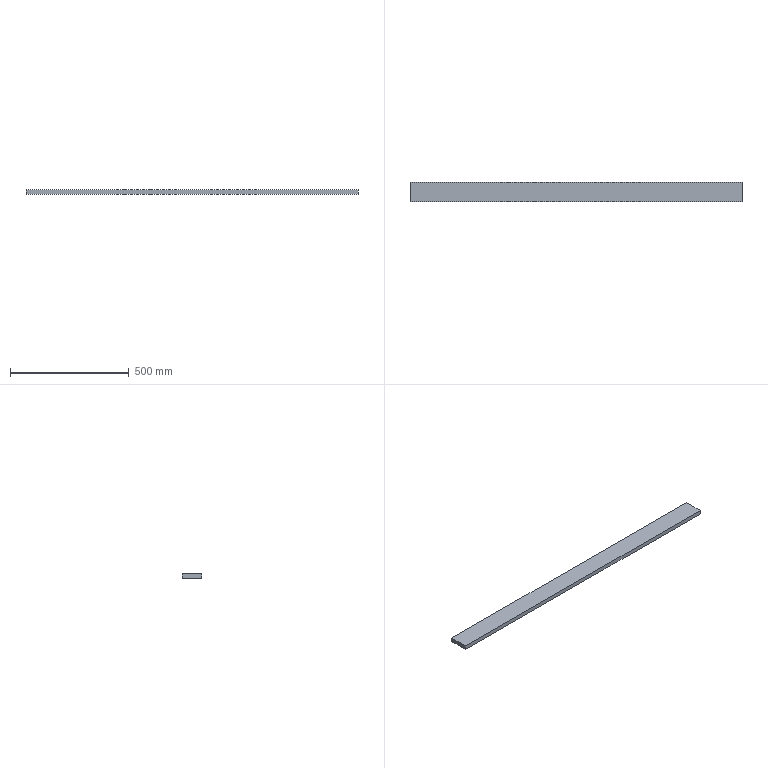Part | STEP file | Frame_right | 1 solid | 6 faces | box 1400 x 82 x 18 mm | volume 2066400 mm3 | plane 6
STEP:
#1=CARTESIAN_POINT('',(0.,0.,0.));
#2=DIRECTION('',(0.,0.,1.));
#3=DIRECTION('',(1.,0.,0.));
#4=AXIS2_PLACEMENT_3D('',#1,#2,#3);
#5=CARTESIAN_POINT('',(-700.,41.,0.));
#6=VERTEX_POINT('',#5);
#7=CARTESIAN_POINT('',(-700.,41.,18.));
#8=VERTEX_POINT('',#7);
#9=CARTESIAN_POINT('',(-700.,41.,0.));
#10=DIRECTION('',(0.,0.,1.));
#11=VECTOR('',#10,1.);
#12=LINE('',#9,#11);
#13=CARTESIAN_POINT('',(-700.,41.,0.));
#14=DIRECTION('',(1.,0.,0.));
#15=DIRECTION('',(0.,-1.,0.));
#16=AXIS2_PLACEMENT_3D('',#13,#14,#15);
#17=PLANE('',#16);
#18=CARTESIAN_POINT('',(0.,0.));
#19=DIRECTION('',(0.,-1.));
#20=VECTOR('',#19,1.);
#21=LINE('',#18,#20);
#22=(GEOMETRIC_REPRESENTATION_CONTEXT(2)PARAMETRIC_REPRESENTATION_CONTEXT()REPRESENTATION_CONTEXT('',''));
#23=DEFINITIONAL_REPRESENTATION('',(#21),#22);
#24=PCURVE('',#17,#23);
#25=CARTESIAN_POINT('',(700.,41.,0.));
#26=DIRECTION('',(0.,-1.,0.));
#27=DIRECTION('',(-1.,0.,0.));
#28=AXIS2_PLACEMENT_3D('',#25,#26,#27);
#29=PLANE('',#28);
#30=CARTESIAN_POINT('',(1400.,0.));
#31=DIRECTION('',(0.,-1.));
#32=VECTOR('',#31,1.);
#33=LINE('',#30,#32);
#34=(GEOMETRIC_REPRESENTATION_CONTEXT(2)PARAMETRIC_REPRESENTATION_CONTEXT()REPRESENTATION_CONTEXT('',''));
#35=DEFINITIONAL_REPRESENTATION('',(#33),#34);
#36=PCURVE('',#29,#35);
#37=SURFACE_CURVE('',#12,(#24,#36),.PCURVE_S1.);
#38=EDGE_CURVE('',#6,#8,#37,.T.);
#39=ORIENTED_EDGE('',*,*,#38,.T.);
#40=CARTESIAN_POINT('',(-700.,-41.,18.));
#41=VERTEX_POINT('',#40);
#42=CARTESIAN_POINT('',(-700.,41.,18.));
#43=DIRECTION('',(0.,-1.,0.));
#44=VECTOR('',#43,1.);
#45=LINE('',#42,#44);
#46=CARTESIAN_POINT('',(0.,-18.));
#47=DIRECTION('',(1.,0.));
#48=VECTOR('',#47,1.);
#49=LINE('',#46,#48);
#50=(GEOMETRIC_REPRESENTATION_CONTEXT(2)PARAMETRIC_REPRESENTATION_CONTEXT()REPRESENTATION_CONTEXT('',''));
#51=DEFINITIONAL_REPRESENTATION('',(#49),#50);
#52=PCURVE('',#17,#51);
#53=CARTESIAN_POINT('',(0.,0.,18.));
#54=DIRECTION('',(0.,0.,1.));
#55=DIRECTION('',(1.,0.,0.));
#56=AXIS2_PLACEMENT_3D('',#53,#54,#55);
#57=PLANE('',#56);
#58=CARTESIAN_POINT('',(-700.,41.));
#59=DIRECTION('',(0.,-1.));
#60=VECTOR('',#59,1.);
#61=LINE('',#58,#60);
#62=(GEOMETRIC_REPRESENTATION_CONTEXT(2)PARAMETRIC_REPRESENTATION_CONTEXT()REPRESENTATION_CONTEXT('',''));
#63=DEFINITIONAL_REPRESENTATION('',(#61),#62);
#64=PCURVE('',#57,#63);
#65=SURFACE_CURVE('',#45,(#52,#64),.PCURVE_S1.);
#66=EDGE_CURVE('',#8,#41,#65,.T.);
#67=ORIENTED_EDGE('',*,*,#66,.T.);
#68=CARTESIAN_POINT('',(-700.,-41.,0.));
#69=VERTEX_POINT('',#68);
#70=CARTESIAN_POINT('',(-700.,-41.,0.));
#71=DIRECTION('',(0.,0.,1.));
#72=VECTOR('',#71,1.);
#73=LINE('',#70,#72);
#74=CARTESIAN_POINT('',(82.,0.));
#75=DIRECTION('',(0.,-1.));
#76=VECTOR('',#75,1.);
#77=LINE('',#74,#76);
#78=(GEOMETRIC_REPRESENTATION_CONTEXT(2)PARAMETRIC_REPRESENTATION_CONTEXT()REPRESENTATION_CONTEXT('',''));
#79=DEFINITIONAL_REPRESENTATION('',(#77),#78);
#80=PCURVE('',#17,#79);
#81=CARTESIAN_POINT('',(-700.,-41.,0.));
#82=DIRECTION('',(0.,1.,0.));
#83=DIRECTION('',(1.,0.,0.));
#84=AXIS2_PLACEMENT_3D('',#81,#82,#83);
#85=PLANE('',#84);
#86=CARTESIAN_POINT('',(0.,0.));
#87=DIRECTION('',(0.,-1.));
#88=VECTOR('',#87,1.);
#89=LINE('',#86,#88);
#90=(GEOMETRIC_REPRESENTATION_CONTEXT(2)PARAMETRIC_REPRESENTATION_CONTEXT()REPRESENTATION_CONTEXT('',''));
#91=DEFINITIONAL_REPRESENTATION('',(#89),#90);
#92=PCURVE('',#85,#91);
#93=SURFACE_CURVE('',#73,(#80,#92),.PCURVE_S1.);
#94=EDGE_CURVE('',#69,#41,#93,.T.);
#95=ORIENTED_EDGE('',*,*,#94,.F.);
#96=CARTESIAN_POINT('',(-700.,41.,0.));
#97=DIRECTION('',(0.,-1.,0.));
#98=VECTOR('',#97,1.);
#99=LINE('',#96,#98);
#100=CARTESIAN_POINT('',(0.,0.));
#101=DIRECTION('',(1.,0.));
#102=VECTOR('',#101,1.);
#103=LINE('',#100,#102);
#104=(GEOMETRIC_REPRESENTATION_CONTEXT(2)PARAMETRIC_REPRESENTATION_CONTEXT()REPRESENTATION_CONTEXT('',''));
#105=DEFINITIONAL_REPRESENTATION('',(#103),#104);
#106=PCURVE('',#17,#105);
#107=CARTESIAN_POINT('',(0.,0.,0.));
#108=DIRECTION('',(0.,0.,1.));
#109=DIRECTION('',(1.,0.,0.));
#110=AXIS2_PLACEMENT_3D('',#107,#108,#109);
#111=PLANE('',#110);
#112=CARTESIAN_POINT('',(-700.,41.));
#113=DIRECTION('',(0.,-1.));
#114=VECTOR('',#113,1.);
#115=LINE('',#112,#114);
#116=(GEOMETRIC_REPRESENTATION_CONTEXT(2)PARAMETRIC_REPRESENTATION_CONTEXT()REPRESENTATION_CONTEXT('',''));
#117=DEFINITIONAL_REPRESENTATION('',(#115),#116);
#118=PCURVE('',#111,#117);
#119=SURFACE_CURVE('',#99,(#106,#118),.PCURVE_S1.);
#120=EDGE_CURVE('',#6,#69,#119,.T.);
#121=ORIENTED_EDGE('',*,*,#120,.F.);
#122=EDGE_LOOP('',(#39,#67,#95,#121));
#123=FACE_BOUND('',#122,.F.);
#124=ADVANCED_FACE('',(#123),#17,.F.);
#125=ORIENTED_EDGE('',*,*,#94,.T.);
#126=CARTESIAN_POINT('',(700.,-41.,18.));
#127=VERTEX_POINT('',#126);
#128=CARTESIAN_POINT('',(-700.,-41.,18.));
#129=DIRECTION('',(1.,0.,0.));
#130=VECTOR('',#129,1.);
#131=LINE('',#128,#130);
#132=CARTESIAN_POINT('',(0.,-18.));
#133=DIRECTION('',(1.,0.));
#134=VECTOR('',#133,1.);
#135=LINE('',#132,#134);
#136=(GEOMETRIC_REPRESENTATION_CONTEXT(2)PARAMETRIC_REPRESENTATION_CONTEXT()REPRESENTATION_CONTEXT('',''));
#137=DEFINITIONAL_REPRESENTATION('',(#135),#136);
#138=PCURVE('',#85,#137);
#139=CARTESIAN_POINT('',(-700.,-41.));
#140=DIRECTION('',(1.,0.));
#141=VECTOR('',#140,1.);
#142=LINE('',#139,#141);
#143=(GEOMETRIC_REPRESENTATION_CONTEXT(2)PARAMETRIC_REPRESENTATION_CONTEXT()REPRESENTATION_CONTEXT('',''));
#144=DEFINITIONAL_REPRESENTATION('',(#142),#143);
#145=PCURVE('',#57,#144);
#146=SURFACE_CURVE('',#131,(#138,#145),.PCURVE_S1.);
#147=EDGE_CURVE('',#41,#127,#146,.T.);
#148=ORIENTED_EDGE('',*,*,#147,.T.);
#149=CARTESIAN_POINT('',(700.,-41.,0.));
#150=VERTEX_POINT('',#149);
#151=CARTESIAN_POINT('',(700.,-41.,0.));
#152=DIRECTION('',(0.,0.,1.));
#153=VECTOR('',#152,1.);
#154=LINE('',#151,#153);
#155=CARTESIAN_POINT('',(1400.,0.));
#156=DIRECTION('',(0.,-1.));
#157=VECTOR('',#156,1.);
#158=LINE('',#155,#157);
#159=(GEOMETRIC_REPRESENTATION_CONTEXT(2)PARAMETRIC_REPRESENTATION_CONTEXT()REPRESENTATION_CONTEXT('',''));
#160=DEFINITIONAL_REPRESENTATION('',(#158),#159);
#161=PCURVE('',#85,#160);
#162=CARTESIAN_POINT('',(700.,-41.,0.));
#163=DIRECTION('',(-1.,0.,0.));
#164=DIRECTION('',(0.,1.,0.));
#165=AXIS2_PLACEMENT_3D('',#162,#163,#164);
#166=PLANE('',#165);
#167=CARTESIAN_POINT('',(0.,0.));
#168=DIRECTION('',(0.,-1.));
#169=VECTOR('',#168,1.);
#170=LINE('',#167,#169);
#171=(GEOMETRIC_REPRESENTATION_CONTEXT(2)PARAMETRIC_REPRESENTATION_CONTEXT()REPRESENTATION_CONTEXT('',''));
#172=DEFINITIONAL_REPRESENTATION('',(#170),#171);
#173=PCURVE('',#166,#172);
#174=SURFACE_CURVE('',#154,(#161,#173),.PCURVE_S1.);
#175=EDGE_CURVE('',#150,#127,#174,.T.);
#176=ORIENTED_EDGE('',*,*,#175,.F.);
#177=CARTESIAN_POINT('',(-700.,-41.,0.));
#178=DIRECTION('',(1.,0.,0.));
#179=VECTOR('',#178,1.);
#180=LINE('',#177,#179);
#181=CARTESIAN_POINT('',(0.,0.));
#182=DIRECTION('',(1.,0.));
#183=VECTOR('',#182,1.);
#184=LINE('',#181,#183);
#185=(GEOMETRIC_REPRESENTATION_CONTEXT(2)PARAMETRIC_REPRESENTATION_CONTEXT()REPRESENTATION_CONTEXT('',''));
#186=DEFINITIONAL_REPRESENTATION('',(#184),#185);
#187=PCURVE('',#85,#186);
#188=CARTESIAN_POINT('',(-700.,-41.));
#189=DIRECTION('',(1.,0.));
#190=VECTOR('',#189,1.);
#191=LINE('',#188,#190);
#192=(GEOMETRIC_REPRESENTATION_CONTEXT(2)PARAMETRIC_REPRESENTATION_CONTEXT()REPRESENTATION_CONTEXT('',''));
#193=DEFINITIONAL_REPRESENTATION('',(#191),#192);
#194=PCURVE('',#111,#193);
#195=SURFACE_CURVE('',#180,(#187,#194),.PCURVE_S1.);
#196=EDGE_CURVE('',#69,#150,#195,.T.);
#197=ORIENTED_EDGE('',*,*,#196,.F.);
#198=EDGE_LOOP('',(#125,#148,#176,#197));
#199=FACE_BOUND('',#198,.F.);
#200=ADVANCED_FACE('',(#199),#85,.F.);
#201=ORIENTED_EDGE('',*,*,#175,.T.);
#202=CARTESIAN_POINT('',(700.,41.,18.));
#203=VERTEX_POINT('',#202);
#204=CARTESIAN_POINT('',(700.,-41.,18.));
#205=DIRECTION('',(0.,1.,0.));
#206=VECTOR('',#205,1.);
#207=LINE('',#204,#206);
#208=CARTESIAN_POINT('',(0.,-18.));
#209=DIRECTION('',(1.,0.));
#210=VECTOR('',#209,1.);
#211=LINE('',#208,#210);
#212=(GEOMETRIC_REPRESENTATION_CONTEXT(2)PARAMETRIC_REPRESENTATION_CONTEXT()REPRESENTATION_CONTEXT('',''));
#213=DEFINITIONAL_REPRESENTATION('',(#211),#212);
#214=PCURVE('',#166,#213);
#215=CARTESIAN_POINT('',(700.,-41.));
#216=DIRECTION('',(0.,1.));
#217=VECTOR('',#216,1.);
#218=LINE('',#215,#217);
#219=(GEOMETRIC_REPRESENTATION_CONTEXT(2)PARAMETRIC_REPRESENTATION_CONTEXT()REPRESENTATION_CONTEXT('',''));
#220=DEFINITIONAL_REPRESENTATION('',(#218),#219);
#221=PCURVE('',#57,#220);
#222=SURFACE_CURVE('',#207,(#214,#221),.PCURVE_S1.);
#223=EDGE_CURVE('',#127,#203,#222,.T.);
#224=ORIENTED_EDGE('',*,*,#223,.T.);
#225=CARTESIAN_POINT('',(700.,41.,0.));
#226=VERTEX_POINT('',#225);
#227=CARTESIAN_POINT('',(700.,41.,0.));
#228=DIRECTION('',(0.,0.,1.));
#229=VECTOR('',#228,1.);
#230=LINE('',#227,#229);
#231=CARTESIAN_POINT('',(82.,0.));
#232=DIRECTION('',(0.,-1.));
#233=VECTOR('',#232,1.);
#234=LINE('',#231,#233);
#235=(GEOMETRIC_REPRESENTATION_CONTEXT(2)PARAMETRIC_REPRESENTATION_CONTEXT()REPRESENTATION_CONTEXT('',''));
#236=DEFINITIONAL_REPRESENTATION('',(#234),#235);
#237=PCURVE('',#166,#236);
#238=CARTESIAN_POINT('',(0.,0.));
#239=DIRECTION('',(0.,-1.));
#240=VECTOR('',#239,1.);
#241=LINE('',#238,#240);
#242=(GEOMETRIC_REPRESENTATION_CONTEXT(2)PARAMETRIC_REPRESENTATION_CONTEXT()REPRESENTATION_CONTEXT('',''));
#243=DEFINITIONAL_REPRESENTATION('',(#241),#242);
#244=PCURVE('',#29,#243);
#245=SURFACE_CURVE('',#230,(#237,#244),.PCURVE_S1.);
#246=EDGE_CURVE('',#226,#203,#245,.T.);
#247=ORIENTED_EDGE('',*,*,#246,.F.);
#248=CARTESIAN_POINT('',(700.,-41.,0.));
#249=DIRECTION('',(0.,1.,0.));
#250=VECTOR('',#249,1.);
#251=LINE('',#248,#250);
#252=CARTESIAN_POINT('',(0.,0.));
#253=DIRECTION('',(1.,0.));
#254=VECTOR('',#253,1.);
#255=LINE('',#252,#254);
#256=(GEOMETRIC_REPRESENTATION_CONTEXT(2)PARAMETRIC_REPRESENTATION_CONTEXT()REPRESENTATION_CONTEXT('',''));
#257=DEFINITIONAL_REPRESENTATION('',(#255),#256);
#258=PCURVE('',#166,#257);
#259=CARTESIAN_POINT('',(700.,-41.));
#260=DIRECTION('',(0.,1.));
#261=VECTOR('',#260,1.);
#262=LINE('',#259,#261);
#263=(GEOMETRIC_REPRESENTATION_CONTEXT(2)PARAMETRIC_REPRESENTATION_CONTEXT()REPRESENTATION_CONTEXT('',''));
#264=DEFINITIONAL_REPRESENTATION('',(#262),#263);
#265=PCURVE('',#111,#264);
#266=SURFACE_CURVE('',#251,(#258,#265),.PCURVE_S1.);
#267=EDGE_CURVE('',#150,#226,#266,.T.);
#268=ORIENTED_EDGE('',*,*,#267,.F.);
#269=EDGE_LOOP('',(#201,#224,#247,#268));
#270=FACE_BOUND('',#269,.F.);
#271=ADVANCED_FACE('',(#270),#166,.F.);
#272=ORIENTED_EDGE('',*,*,#246,.T.);
#273=CARTESIAN_POINT('',(700.,41.,18.));
#274=DIRECTION('',(-1.,0.,0.));
#275=VECTOR('',#274,1.);
#276=LINE('',#273,#275);
#277=CARTESIAN_POINT('',(0.,-18.));
#278=DIRECTION('',(1.,0.));
#279=VECTOR('',#278,1.);
#280=LINE('',#277,#279);
#281=(GEOMETRIC_REPRESENTATION_CONTEXT(2)PARAMETRIC_REPRESENTATION_CONTEXT()REPRESENTATION_CONTEXT('',''));
#282=DEFINITIONAL_REPRESENTATION('',(#280),#281);
#283=PCURVE('',#29,#282);
#284=CARTESIAN_POINT('',(700.,41.));
#285=DIRECTION('',(-1.,0.));
#286=VECTOR('',#285,1.);
#287=LINE('',#284,#286);
#288=(GEOMETRIC_REPRESENTATION_CONTEXT(2)PARAMETRIC_REPRESENTATION_CONTEXT()REPRESENTATION_CONTEXT('',''));
#289=DEFINITIONAL_REPRESENTATION('',(#287),#288);
#290=PCURVE('',#57,#289);
#291=SURFACE_CURVE('',#276,(#283,#290),.PCURVE_S1.);
#292=EDGE_CURVE('',#203,#8,#291,.T.);
#293=ORIENTED_EDGE('',*,*,#292,.T.);
#294=ORIENTED_EDGE('',*,*,#38,.F.);
#295=CARTESIAN_POINT('',(700.,41.,0.));
#296=DIRECTION('',(-1.,0.,0.));
#297=VECTOR('',#296,1.);
#298=LINE('',#295,#297);
#299=CARTESIAN_POINT('',(0.,0.));
#300=DIRECTION('',(1.,0.));
#301=VECTOR('',#300,1.);
#302=LINE('',#299,#301);
#303=(GEOMETRIC_REPRESENTATION_CONTEXT(2)PARAMETRIC_REPRESENTATION_CONTEXT()REPRESENTATION_CONTEXT('',''));
#304=DEFINITIONAL_REPRESENTATION('',(#302),#303);
#305=PCURVE('',#29,#304);
#306=CARTESIAN_POINT('',(700.,41.));
#307=DIRECTION('',(-1.,0.));
#308=VECTOR('',#307,1.);
#309=LINE('',#306,#308);
#310=(GEOMETRIC_REPRESENTATION_CONTEXT(2)PARAMETRIC_REPRESENTATION_CONTEXT()REPRESENTATION_CONTEXT('',''));
#311=DEFINITIONAL_REPRESENTATION('',(#309),#310);
#312=PCURVE('',#111,#311);
#313=SURFACE_CURVE('',#298,(#305,#312),.PCURVE_S1.);
#314=EDGE_CURVE('',#226,#6,#313,.T.);
#315=ORIENTED_EDGE('',*,*,#314,.F.);
#316=EDGE_LOOP('',(#272,#293,#294,#315));
#317=FACE_BOUND('',#316,.F.);
#318=ADVANCED_FACE('',(#317),#29,.F.);
#319=ORIENTED_EDGE('',*,*,#120,.T.);
#320=ORIENTED_EDGE('',*,*,#196,.T.);
#321=ORIENTED_EDGE('',*,*,#267,.T.);
#322=ORIENTED_EDGE('',*,*,#314,.T.);
#323=EDGE_LOOP('',(#319,#320,#321,#322));
#324=FACE_BOUND('',#323,.F.);
#325=ADVANCED_FACE('',(#324),#111,.F.);
#326=ORIENTED_EDGE('',*,*,#66,.T.);
#327=ORIENTED_EDGE('',*,*,#147,.T.);
#328=ORIENTED_EDGE('',*,*,#223,.T.);
#329=ORIENTED_EDGE('',*,*,#292,.T.);
#330=EDGE_LOOP('',(#326,#327,#328,#329));
#331=FACE_BOUND('',#330,.T.);
#332=ADVANCED_FACE('',(#331),#57,.T.);
#333=CLOSED_SHELL('',(#124,#200,#271,#318,#325,#332));
#334=MANIFOLD_SOLID_BREP('',#333);
#335=(LENGTH_UNIT()NAMED_UNIT(*)SI_UNIT(.MILLI.,.METRE.));
#336=UNCERTAINTY_MEASURE_WITH_UNIT(LENGTH_MEASURE(0.0000001),#335,'','');
#337=(NAMED_UNIT(*)PLANE_ANGLE_UNIT()SI_UNIT($,.RADIAN.));
#338=(NAMED_UNIT(*)SI_UNIT($,.STERADIAN.)SOLID_ANGLE_UNIT());
#339=(GEOMETRIC_REPRESENTATION_CONTEXT(3)GLOBAL_UNCERTAINTY_ASSIGNED_CONTEXT((#336))GLOBAL_UNIT_ASSIGNED_CONTEXT((#335,#337,#338))REPRESENTATION_CONTEXT('',''));
#340=ADVANCED_BREP_SHAPE_REPRESENTATION('',(#4,#334),#339);